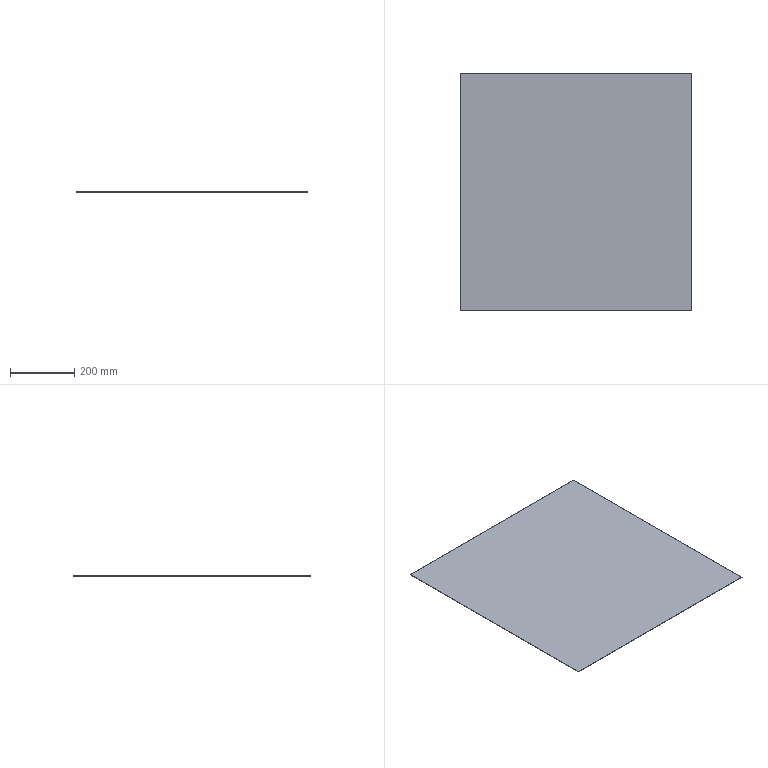Part | STEP file | Guide wheel mechanism revised.sldasm-Part-170 | 1 solid | 6 faces | box 720 x 740 x 1.2 mm | volume 639360 mm3 | plane 6
STEP:
#1=CARTESIAN_POINT('',(-360.,740.,-260.));
#2=VERTEX_POINT('',#1);
#3=CARTESIAN_POINT('',(-360.,0.,-260.));
#4=VERTEX_POINT('',#3);
#5=CARTESIAN_POINT('',(-360.,740.,-260.));
#6=DIRECTION('',(0.,-1.,0.));
#7=VECTOR('',#6,1000.);
#8=LINE('',#5,#7);
#9=EDGE_CURVE('',#2,#4,#8,.T.);
#10=ORIENTED_EDGE('',*,*,#9,.T.);
#11=CARTESIAN_POINT('',(-360.,0.,-258.8));
#12=VERTEX_POINT('',#11);
#13=CARTESIAN_POINT('',(-360.,0.,-258.8));
#14=DIRECTION('',(0.,0.,-1.));
#15=VECTOR('',#14,1000.);
#16=LINE('',#13,#15);
#17=EDGE_CURVE('',#12,#4,#16,.T.);
#18=ORIENTED_EDGE('',*,*,#17,.F.);
#19=CARTESIAN_POINT('',(-360.,740.,-258.8));
#20=VERTEX_POINT('',#19);
#21=CARTESIAN_POINT('',(-360.,740.,-258.8));
#22=DIRECTION('',(0.,-1.,0.));
#23=VECTOR('',#22,1000.);
#24=LINE('',#21,#23);
#25=EDGE_CURVE('',#20,#12,#24,.T.);
#26=ORIENTED_EDGE('',*,*,#25,.F.);
#27=CARTESIAN_POINT('',(-360.,740.,-258.8));
#28=DIRECTION('',(0.,0.,-1.));
#29=VECTOR('',#28,1000.);
#30=LINE('',#27,#29);
#31=EDGE_CURVE('',#20,#2,#30,.T.);
#32=ORIENTED_EDGE('',*,*,#31,.T.);
#33=EDGE_LOOP('',(#10,#18,#26,#32));
#34=FACE_OUTER_BOUND('',#33,.T.);
#35=CARTESIAN_POINT('',(-360.,740.,-258.8));
#36=DIRECTION('',(1.,0.,0.));
#37=DIRECTION('',(0.,1.,0.));
#38=AXIS2_PLACEMENT_3D('',#35,#36,#37);
#39=PLANE('',#38);
#40=ADVANCED_FACE('',(#34),#39,.F.);
#41=CARTESIAN_POINT('',(360.,0.,-260.));
#42=VERTEX_POINT('',#41);
#43=CARTESIAN_POINT('',(-360.,0.,-260.));
#44=DIRECTION('',(1.,0.,0.));
#45=VECTOR('',#44,1000.);
#46=LINE('',#43,#45);
#47=EDGE_CURVE('',#4,#42,#46,.T.);
#48=ORIENTED_EDGE('',*,*,#47,.T.);
#49=CARTESIAN_POINT('',(360.,0.,-258.8));
#50=VERTEX_POINT('',#49);
#51=CARTESIAN_POINT('',(360.,0.,-258.8));
#52=DIRECTION('',(0.,0.,-1.));
#53=VECTOR('',#52,1000.);
#54=LINE('',#51,#53);
#55=EDGE_CURVE('',#50,#42,#54,.T.);
#56=ORIENTED_EDGE('',*,*,#55,.F.);
#57=CARTESIAN_POINT('',(-360.,0.,-258.8));
#58=DIRECTION('',(1.,0.,0.));
#59=VECTOR('',#58,1000.);
#60=LINE('',#57,#59);
#61=EDGE_CURVE('',#12,#50,#60,.T.);
#62=ORIENTED_EDGE('',*,*,#61,.F.);
#63=ORIENTED_EDGE('',*,*,#17,.T.);
#64=EDGE_LOOP('',(#48,#56,#62,#63));
#65=FACE_OUTER_BOUND('',#64,.T.);
#66=CARTESIAN_POINT('',(-360.,0.,-258.8));
#67=DIRECTION('',(0.,1.,0.));
#68=DIRECTION('',(0.,0.,1.));
#69=AXIS2_PLACEMENT_3D('',#66,#67,#68);
#70=PLANE('',#69);
#71=ADVANCED_FACE('',(#65),#70,.F.);
#72=CARTESIAN_POINT('',(360.,740.,-260.));
#73=VERTEX_POINT('',#72);
#74=CARTESIAN_POINT('',(360.,740.,-260.));
#75=DIRECTION('',(0.,1.,0.));
#76=VECTOR('',#75,1000.);
#77=LINE('',#74,#76);
#78=EDGE_CURVE('',#42,#73,#77,.T.);
#79=ORIENTED_EDGE('',*,*,#78,.T.);
#80=CARTESIAN_POINT('',(360.,740.,-258.8));
#81=VERTEX_POINT('',#80);
#82=CARTESIAN_POINT('',(360.,740.,-258.8));
#83=DIRECTION('',(0.,0.,-1.));
#84=VECTOR('',#83,1000.);
#85=LINE('',#82,#84);
#86=EDGE_CURVE('',#81,#73,#85,.T.);
#87=ORIENTED_EDGE('',*,*,#86,.F.);
#88=CARTESIAN_POINT('',(360.,740.,-258.8));
#89=DIRECTION('',(0.,1.,0.));
#90=VECTOR('',#89,1000.);
#91=LINE('',#88,#90);
#92=EDGE_CURVE('',#50,#81,#91,.T.);
#93=ORIENTED_EDGE('',*,*,#92,.F.);
#94=ORIENTED_EDGE('',*,*,#55,.T.);
#95=EDGE_LOOP('',(#79,#87,#93,#94));
#96=FACE_OUTER_BOUND('',#95,.T.);
#97=CARTESIAN_POINT('',(360.,740.,-258.8));
#98=DIRECTION('',(-1.,0.,0.));
#99=DIRECTION('',(0.,-1.,0.));
#100=AXIS2_PLACEMENT_3D('',#97,#98,#99);
#101=PLANE('',#100);
#102=ADVANCED_FACE('',(#96),#101,.F.);
#103=CARTESIAN_POINT('',(-360.,740.,-260.));
#104=DIRECTION('',(-1.,0.,0.));
#105=VECTOR('',#104,1000.);
#106=LINE('',#103,#105);
#107=EDGE_CURVE('',#73,#2,#106,.T.);
#108=ORIENTED_EDGE('',*,*,#107,.T.);
#109=ORIENTED_EDGE('',*,*,#31,.F.);
#110=CARTESIAN_POINT('',(-360.,740.,-258.8));
#111=DIRECTION('',(-1.,0.,0.));
#112=VECTOR('',#111,1000.);
#113=LINE('',#110,#112);
#114=EDGE_CURVE('',#81,#20,#113,.T.);
#115=ORIENTED_EDGE('',*,*,#114,.F.);
#116=ORIENTED_EDGE('',*,*,#86,.T.);
#117=EDGE_LOOP('',(#108,#109,#115,#116));
#118=FACE_OUTER_BOUND('',#117,.T.);
#119=CARTESIAN_POINT('',(-360.,740.,-258.8));
#120=DIRECTION('',(0.,-1.,0.));
#121=DIRECTION('',(0.,0.,-1.));
#122=AXIS2_PLACEMENT_3D('',#119,#120,#121);
#123=PLANE('',#122);
#124=ADVANCED_FACE('',(#118),#123,.F.);
#125=ORIENTED_EDGE('',*,*,#25,.T.);
#126=ORIENTED_EDGE('',*,*,#61,.T.);
#127=ORIENTED_EDGE('',*,*,#92,.T.);
#128=ORIENTED_EDGE('',*,*,#114,.T.);
#129=EDGE_LOOP('',(#125,#126,#127,#128));
#130=FACE_OUTER_BOUND('',#129,.T.);
#131=CARTESIAN_POINT('',(0.,0.,-258.8));
#132=DIRECTION('',(0.,0.,1.));
#133=DIRECTION('',(1.,0.,0.));
#134=AXIS2_PLACEMENT_3D('',#131,#132,#133);
#135=PLANE('',#134);
#136=ADVANCED_FACE('',(#130),#135,.T.);
#137=ORIENTED_EDGE('',*,*,#9,.F.);
#138=ORIENTED_EDGE('',*,*,#107,.F.);
#139=ORIENTED_EDGE('',*,*,#78,.F.);
#140=ORIENTED_EDGE('',*,*,#47,.F.);
#141=EDGE_LOOP('',(#137,#138,#139,#140));
#142=FACE_OUTER_BOUND('',#141,.T.);
#143=CARTESIAN_POINT('',(0.,0.,-260.));
#144=DIRECTION('',(0.,0.,1.));
#145=DIRECTION('',(1.,0.,0.));
#146=AXIS2_PLACEMENT_3D('',#143,#144,#145);
#147=PLANE('',#146);
#148=ADVANCED_FACE('',(#142),#147,.F.);
#149=CLOSED_SHELL('',(#40,#71,#102,#124,#136,#148));
#150=MANIFOLD_SOLID_BREP('',#149);
#151=CARTESIAN_POINT('',(0.,0.,0.));
#152=DIRECTION('',(0.,0.,1.));
#153=DIRECTION('',(1.,0.,0.));
#154=AXIS2_PLACEMENT_3D('',#151,#152,#153);
#155=(LENGTH_UNIT()NAMED_UNIT(*)SI_UNIT(.MILLI.,.METRE.));
#156=UNCERTAINTY_MEASURE_WITH_UNIT(LENGTH_MEASURE(0.00001),#155,'','');
#157=(NAMED_UNIT(*)PLANE_ANGLE_UNIT()SI_UNIT($,.RADIAN.));
#158=(NAMED_UNIT(*)SI_UNIT($,.STERADIAN.)SOLID_ANGLE_UNIT());
#159=(GEOMETRIC_REPRESENTATION_CONTEXT(3)GLOBAL_UNCERTAINTY_ASSIGNED_CONTEXT((#156))GLOBAL_UNIT_ASSIGNED_CONTEXT((#155,#157,#158))REPRESENTATION_CONTEXT('',''));
#160=ADVANCED_BREP_SHAPE_REPRESENTATION('',(#150,#154),#159);